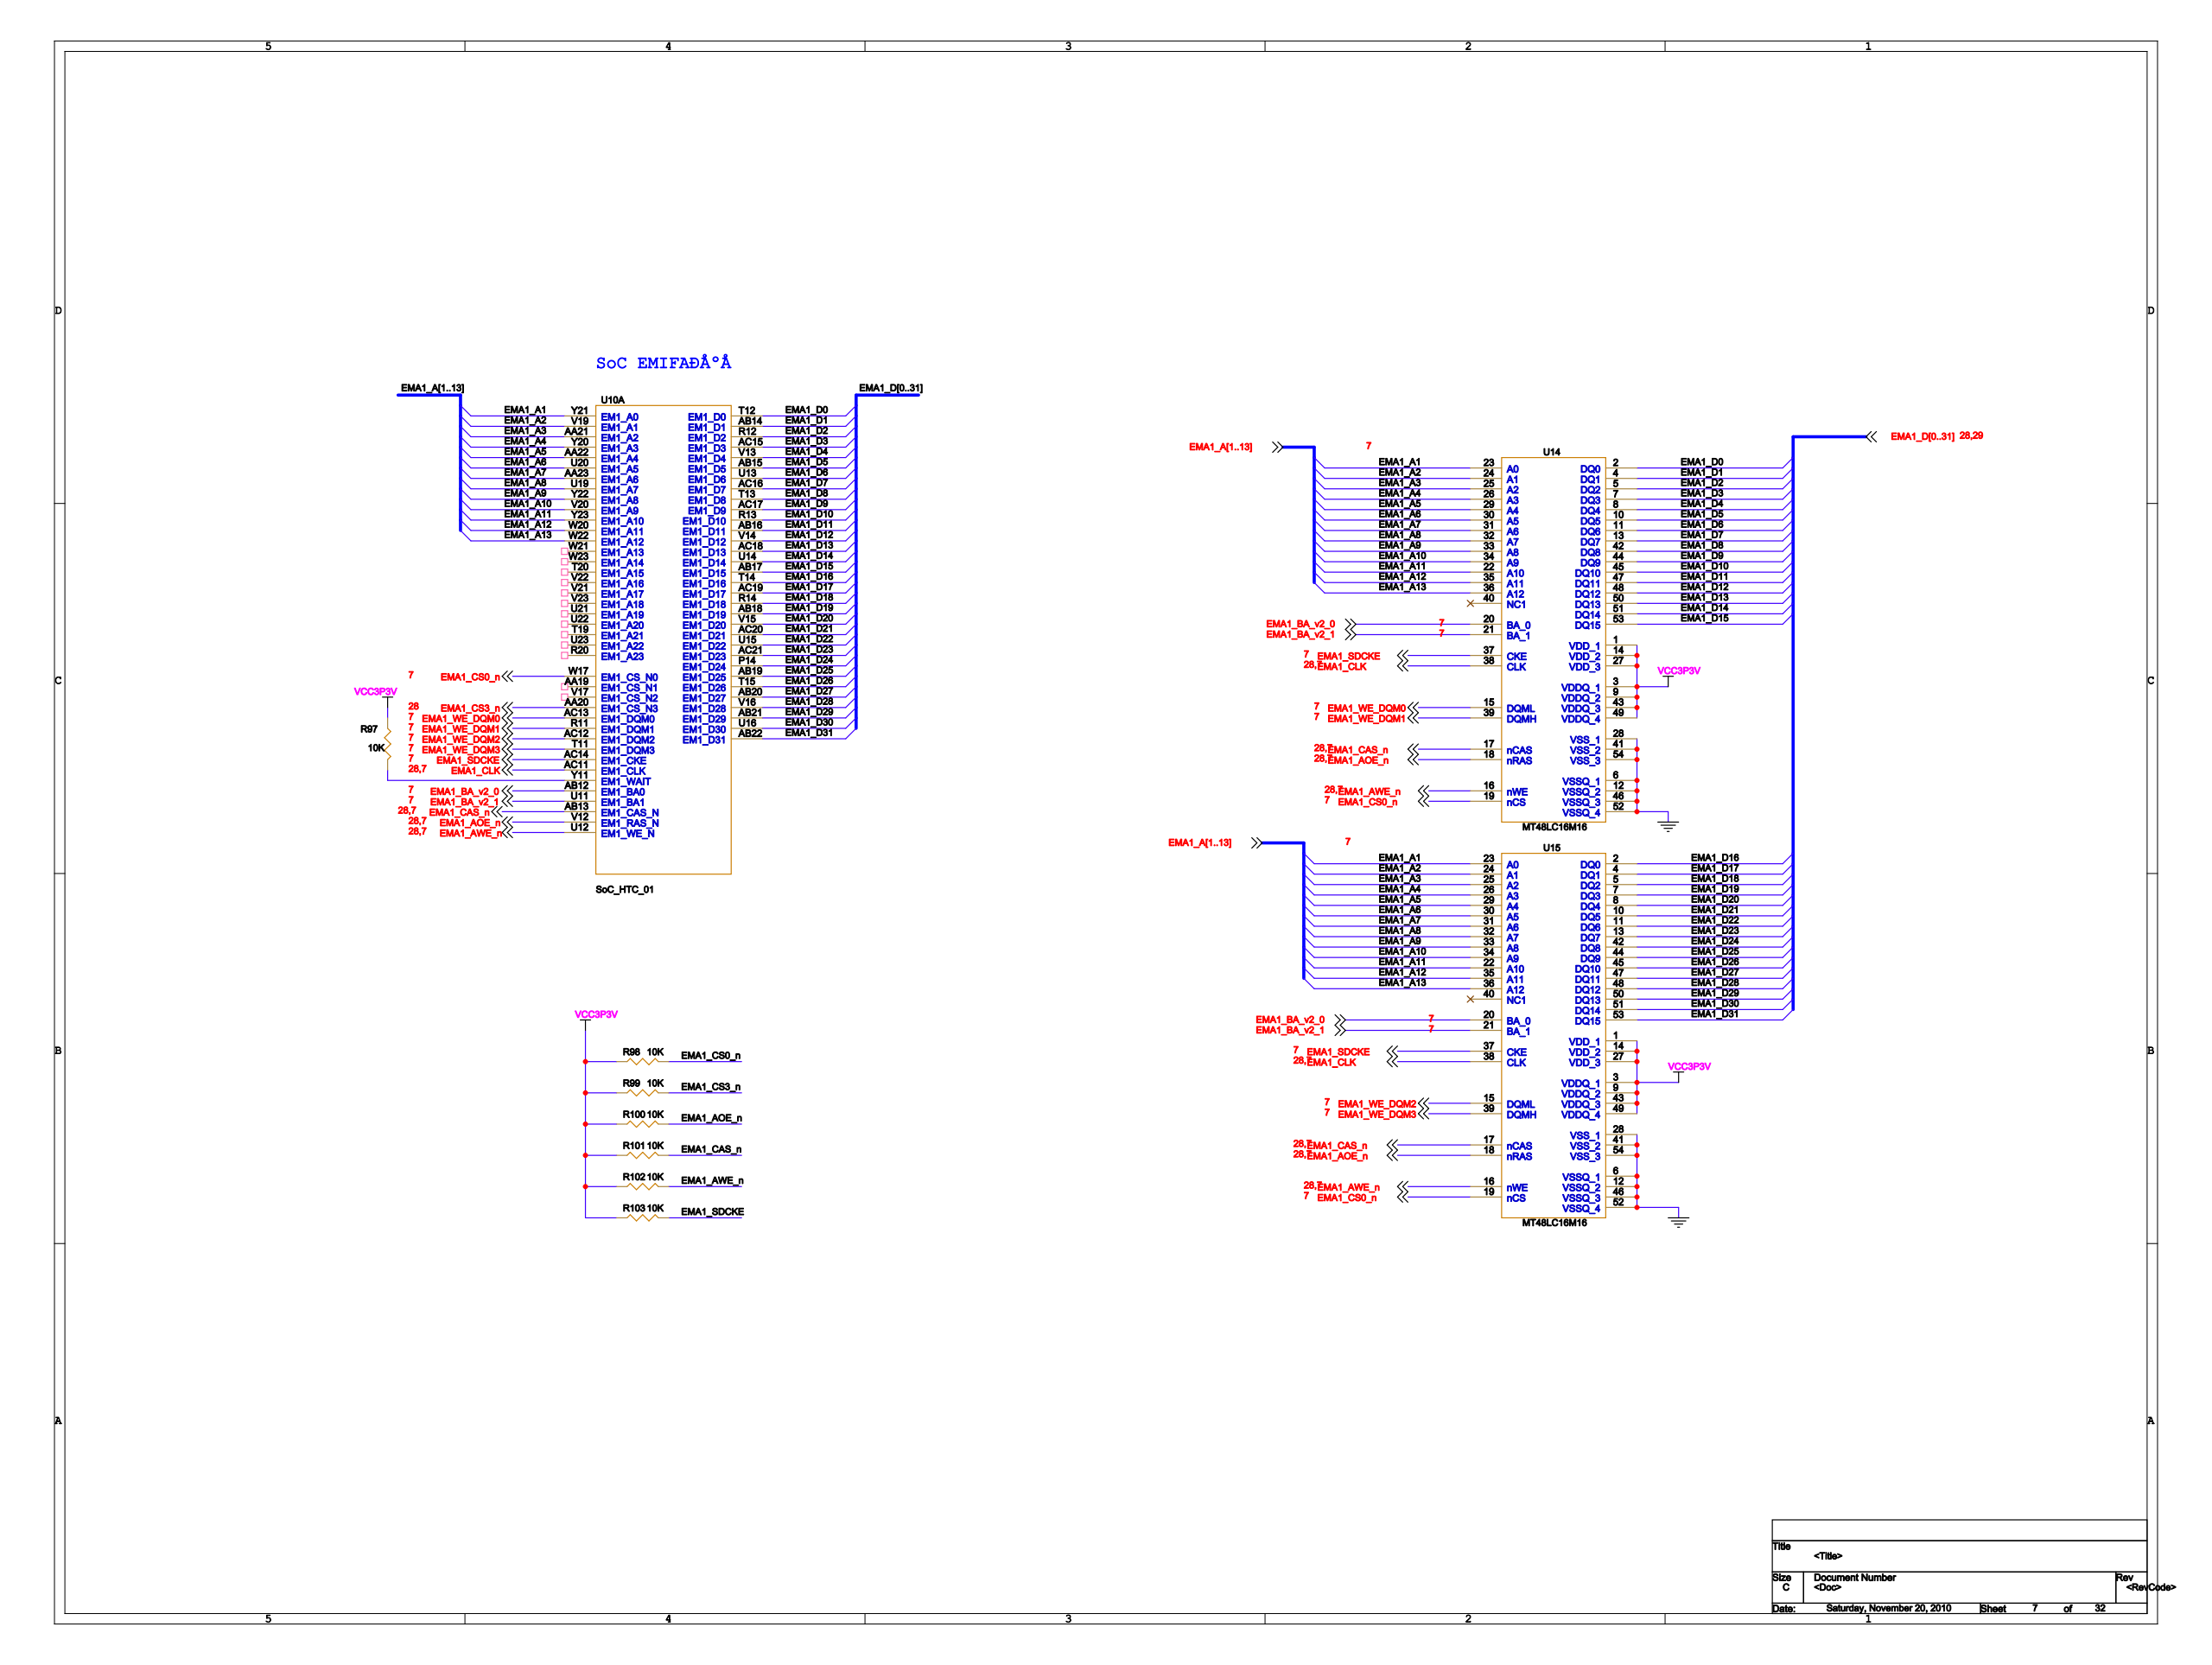Circuit board | Cadence Allegro | 1001 parts | 1318 nets | one sheet of the schematic
Parts on this sheet (reference | value | footprint):
R97 | 10K | 0603
R98 | 10K | 0603
R99 | 10K | 0603
R100 | 10K | 0603
R101 | 10K | 0603
R102 | 10K | 0603
R103 | 10K | 0603
U10 | SoC_HTC_01 | L529_XIN
U11 | MT48LC32M16 | TSOP54
U14 | MT48LC16M16 | TSOP54
U15 | MT48LC16M16 | TSOP54
U20 | MT48LC16M16 | TSOP54
U21 | MT48LC16M16 | TSOP54
U23 | MT48LC32M16 | TSOP54
Nets of these parts (net: part-pin ...):
EMA1_D5: U10-AB15 U14-10
EMA1_D1: U10-AB14 U14-4
EMA1_D3: U10-AC15 U14-7
EMA1_CAS_N: R101-2 U10-AB13 U14-17 U15-17
EMA1_D11: U10-AB16 U14-47
EMA1_D7: U10-AC16 U14-13
EMA1_CLK: U10-AC11 U14-38 U15-38
EMA1_D26: U10-T15 U15-45
EMA1_D8: U10-T13 U14-42
EMA1_D14: U10-U14 U14-51
EMA1_D16: U10-T14 U15-2
EMA1_D24: U10-P14 U15-42
EMA1_D10: U10-R13 U14-45
EMA1_D0: U10-T12 U14-2
EMA1_D18: U10-R14 U15-5
EMA1_D2: U10-R12 U14-5
EMA1_D4: U10-V13 U14-8
EMA1_AWE_N: R102-2 U10-U12 U14-16 U15-16
EMA1_AOE_N: R100-2 U10-V12 U14-18 U15-18
EMA1_D13: U10-AC18 U14-50
EMA1_D23: U10-AC21 U15-13
EMA1_D31: U10-AB22 U15-53
EMA1_D12: U10-V14 U14-48
EMA1_D20: U10-V15 U15-8
EMA1_D22: U10-U15 U15-11
EMA1_D25: U10-AB19 U15-44
EMA1_D21: U10-AC20 U15-10
EMA1_D27: U10-AB20 U15-47
EMA1_CS3_N: R99-2 U10-AA20
EMA1_D6: U10-U13 U14-11
EMA1_D28: U10-V16 U15-48
EMA1_D30: U10-U16 U15-51
EMA1_D19: U10-AB18 U15-7
EMA1_D17: U10-AC19 U15-4
EMA1_D29: U10-AB21 U15-50
EMA1_D15: U10-AB17 U14-53
EMA1_D9: U10-AC17 U14-44
VCC3P3V: R97-2 R98-1 R99-1 R100-1 R101-1 R102-1 R103-1 U11-1 U11-3 U11-9 U11-14 U11-27 U11-43 U11-49 U14-1 U14-3 U14-9 U14-14 U14-27 U14-43 U14-49 U15-1 U15-3 U15-9 U15-14 U15-27 U15-43 U15-49 U20-1 U20-3 U20-9 U20-14 U20-27 U20-43 U20-49 U21-1 U21-3 U21-9 U21-14 U21-27 U21-43 U21-49 U23-1 U23-3 U23-9 U23-14 U23-27 U23-43 U23-49
EMA1_A1: U10-Y21 U14-23 U15-23
EMA1_A2: U10-V19 U14-24 U15-24
EMA1_A11: U10-Y23 U14-22 U15-22
EMA1_A12: U10-W20 U14-35 U15-35
EMA1_A13: U10-W22 U14-36 U15-36
EMA1_A3: U10-AA21 U14-25 U15-25
EMA1_A4: U10-Y20 U14-26 U15-26
EMA1_A5: U10-AA22 U14-29 U15-29
EMA1_A6: U10-U20 U14-30 U15-30
EMA1_A7: U10-AA23 U14-31 U15-31
EMA1_A8: U10-U19 U14-32 U15-32
EMA1_A9: U10-Y22 U14-33 U15-33
EMA1_A10: U10-V20 U14-34 U15-34
EMA1_SDCKE: R103-2 U10-AC14 U14-37 U15-37
EMA1_CS0_N: R98-2 U10-W17 U14-19 U15-19
EMA1_WE_DQM0: U10-AC13 U14-15
EMA1_WE_DQM1: U10-R11 U14-39
EMA1_WE_DQM2: U10-AC12 U15-15
EMA1_WE_DQM3: U10-T11 U15-39
N16742525: R97-1 U10-Y11